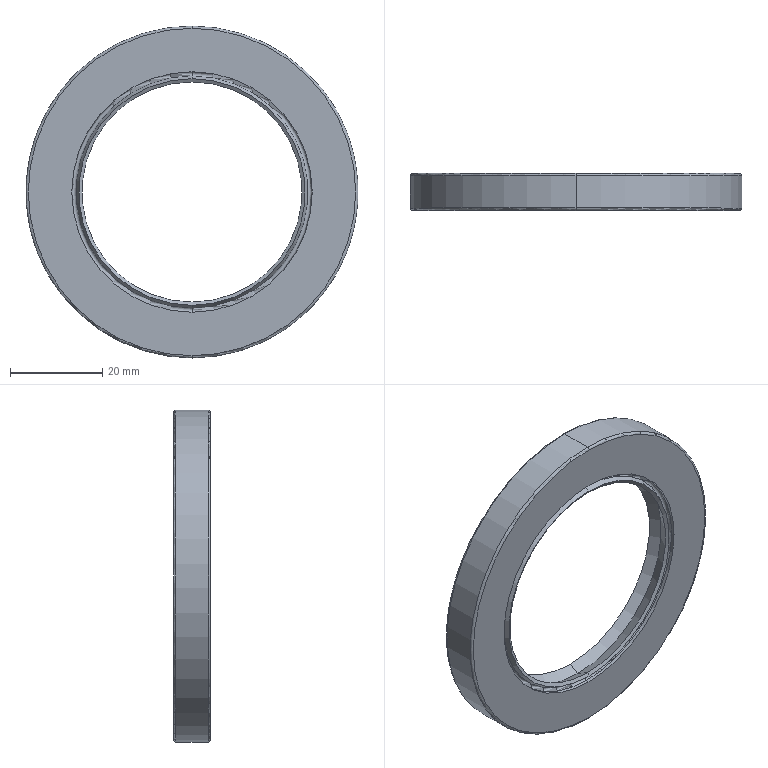Part | SolidWorks | features BaseBody 1 | 1 solid | 36 faces | box 72 x 8 x 72 mm | volume 7067 mm3 | torus 14 | cone 10 | cylinder 8 | plane 4 | commonest cylinder face diameters 52.145 x2 53.98 x2 69 x2 72 x2
STEP:
#1=CARTESIAN_POINT('',(0.,0.,24.573));
#2=VERTEX_POINT('',#1);
#3=CARTESIAN_POINT('',(0.,0.,-24.573));
#4=VERTEX_POINT('',#3);
#5=CARTESIAN_POINT('',(0.,0.,0.));
#6=DIRECTION('',(0.,1.,0.));
#7=DIRECTION('',(0.,0.,1.));
#8=AXIS2_PLACEMENT_3D('',#5,#6,#7);
#9=CIRCLE('',#8,24.573);
#10=EDGE_CURVE('',#2,#4,#9,.T.);
#11=ORIENTED_EDGE('',*,*,#10,.T.);
#12=CARTESIAN_POINT('',(0.,0.9821,-25.14));
#13=VERTEX_POINT('',#12);
#14=CARTESIAN_POINT('',(0.,0.9821,-25.14));
#15=DIRECTION('',(0.,0.866,-0.5));
#16=VECTOR('',#15,1000.);
#17=LINE('',#14,#16);
#18=EDGE_CURVE('',#4,#13,#17,.T.);
#19=ORIENTED_EDGE('',*,*,#18,.T.);
#20=CARTESIAN_POINT('',(0.,0.9821,25.14));
#21=VERTEX_POINT('',#20);
#22=CARTESIAN_POINT('',(0.,0.9821,0.));
#23=DIRECTION('',(0.,1.,0.));
#24=DIRECTION('',(0.,0.,1.));
#25=AXIS2_PLACEMENT_3D('',#22,#23,#24);
#26=CIRCLE('',#25,25.14);
#27=EDGE_CURVE('',#21,#13,#26,.T.);
#28=ORIENTED_EDGE('',*,*,#27,.F.);
#29=CARTESIAN_POINT('',(0.,0.9821,25.14));
#30=DIRECTION('',(0.,0.866,0.5));
#31=VECTOR('',#30,1000.);
#32=LINE('',#29,#31);
#33=EDGE_CURVE('',#2,#21,#32,.T.);
#34=ORIENTED_EDGE('',*,*,#33,.F.);
#35=EDGE_LOOP('',(#11,#19,#28,#34));
#36=FACE_OUTER_BOUND('',#35,.T.);
#37=CARTESIAN_POINT('',(0.,0.9821,0.));
#38=DIRECTION('',(0.,1.,0.));
#39=DIRECTION('',(0.,0.,1.));
#40=AXIS2_PLACEMENT_3D('',#37,#38,#39);
#41=CONICAL_SURFACE('',#40,25.14,0.5236);
#42=ADVANCED_FACE('',(#36),#41,.T.);
#43=CARTESIAN_POINT('',(0.,0.4041,-23.873));
#44=VERTEX_POINT('',#43);
#45=CARTESIAN_POINT('',(0.,0.4041,23.873));
#46=VERTEX_POINT('',#45);
#47=CARTESIAN_POINT('',(0.,0.4041,0.));
#48=DIRECTION('',(0.,1.,0.));
#49=DIRECTION('',(0.,0.,1.));
#50=AXIS2_PLACEMENT_3D('',#47,#48,#49);
#51=CIRCLE('',#50,23.873);
#52=EDGE_CURVE('',#44,#46,#51,.T.);
#53=ORIENTED_EDGE('',*,*,#52,.T.);
#54=CARTESIAN_POINT('',(0.,0.,24.573));
#55=DIRECTION('',(0.,-0.5,0.866));
#56=VECTOR('',#55,1000.);
#57=LINE('',#54,#56);
#58=EDGE_CURVE('',#46,#2,#57,.T.);
#59=ORIENTED_EDGE('',*,*,#58,.T.);
#60=CARTESIAN_POINT('',(0.,0.,0.));
#61=DIRECTION('',(0.,1.,0.));
#62=DIRECTION('',(0.,0.,1.));
#63=AXIS2_PLACEMENT_3D('',#60,#61,#62);
#64=CIRCLE('',#63,24.573);
#65=EDGE_CURVE('',#4,#2,#64,.T.);
#66=ORIENTED_EDGE('',*,*,#65,.F.);
#67=CARTESIAN_POINT('',(0.,0.,-24.573));
#68=DIRECTION('',(0.,-0.5,-0.866));
#69=VECTOR('',#68,1000.);
#70=LINE('',#67,#69);
#71=EDGE_CURVE('',#44,#4,#70,.T.);
#72=ORIENTED_EDGE('',*,*,#71,.F.);
#73=EDGE_LOOP('',(#53,#59,#66,#72));
#74=FACE_OUTER_BOUND('',#73,.T.);
#75=CARTESIAN_POINT('',(0.,0.,0.));
#76=DIRECTION('',(0.,-1.,0.));
#77=DIRECTION('',(0.,0.,-1.));
#78=AXIS2_PLACEMENT_3D('',#75,#76,#77);
#79=CONICAL_SURFACE('',#78,24.573,1.047);
#80=ADVANCED_FACE('',(#74),#79,.F.);
#81=ORIENTED_EDGE('',*,*,#52,.F.);
#82=CARTESIAN_POINT('',(0.,3.472,-25.644));
#83=VERTEX_POINT('',#82);
#84=CARTESIAN_POINT('',(0.,0.4041,-23.873));
#85=DIRECTION('',(0.,0.866,-0.5));
#86=VECTOR('',#85,1000.);
#87=LINE('',#84,#86);
#88=EDGE_CURVE('',#44,#83,#87,.T.);
#89=ORIENTED_EDGE('',*,*,#88,.T.);
#90=CARTESIAN_POINT('',(0.,3.472,25.644));
#91=VERTEX_POINT('',#90);
#92=CARTESIAN_POINT('',(0.,3.472,0.));
#93=DIRECTION('',(0.,1.,0.));
#94=DIRECTION('',(0.,0.,1.));
#95=AXIS2_PLACEMENT_3D('',#92,#93,#94);
#96=CIRCLE('',#95,25.644);
#97=EDGE_CURVE('',#83,#91,#96,.T.);
#98=ORIENTED_EDGE('',*,*,#97,.T.);
#99=CARTESIAN_POINT('',(0.,0.4041,23.873));
#100=DIRECTION('',(0.,0.866,0.5));
#101=VECTOR('',#100,1000.);
#102=LINE('',#99,#101);
#103=EDGE_CURVE('',#46,#91,#102,.T.);
#104=ORIENTED_EDGE('',*,*,#103,.F.);
#105=EDGE_LOOP('',(#81,#89,#98,#104));
#106=FACE_OUTER_BOUND('',#105,.T.);
#107=CARTESIAN_POINT('',(0.,0.4041,0.));
#108=DIRECTION('',(0.,1.,0.));
#109=DIRECTION('',(0.,0.,1.));
#110=AXIS2_PLACEMENT_3D('',#107,#108,#109);
#111=CONICAL_SURFACE('',#110,23.873,0.5236);
#112=ADVANCED_FACE('',(#106),#111,.F.);
#113=CARTESIAN_POINT('',(0.,5.7,-24.25));
#114=VERTEX_POINT('',#113);
#115=CARTESIAN_POINT('',(0.,5.7,24.25));
#116=VERTEX_POINT('',#115);
#117=CARTESIAN_POINT('',(0.,5.7,0.));
#118=DIRECTION('',(0.,1.,0.));
#119=DIRECTION('',(0.,0.,1.));
#120=AXIS2_PLACEMENT_3D('',#117,#118,#119);
#121=CIRCLE('',#120,24.25);
#122=EDGE_CURVE('',#114,#116,#121,.T.);
#123=ORIENTED_EDGE('',*,*,#122,.T.);
#124=CARTESIAN_POINT('',(0.,3.472,25.644));
#125=DIRECTION('',(0.,-0.8478,0.5303));
#126=VECTOR('',#125,1000.);
#127=LINE('',#124,#126);
#128=EDGE_CURVE('',#116,#91,#127,.T.);
#129=ORIENTED_EDGE('',*,*,#128,.T.);
#130=ORIENTED_EDGE('',*,*,#97,.F.);
#131=CARTESIAN_POINT('',(0.,3.472,-25.644));
#132=DIRECTION('',(0.,-0.8478,-0.5303));
#133=VECTOR('',#132,1000.);
#134=LINE('',#131,#133);
#135=EDGE_CURVE('',#114,#83,#134,.T.);
#136=ORIENTED_EDGE('',*,*,#135,.F.);
#137=EDGE_LOOP('',(#123,#129,#130,#136));
#138=FACE_OUTER_BOUND('',#137,.T.);
#139=CARTESIAN_POINT('',(0.,3.472,0.));
#140=DIRECTION('',(0.,-1.,0.));
#141=DIRECTION('',(0.,0.,-1.));
#142=AXIS2_PLACEMENT_3D('',#139,#140,#141);
#143=CONICAL_SURFACE('',#142,25.644,0.5589);
#144=ADVANCED_FACE('',(#138),#143,.F.);
#145=ORIENTED_EDGE('',*,*,#122,.F.);
#146=CARTESIAN_POINT('',(0.,7.,-26.328));
#147=VERTEX_POINT('',#146);
#148=CARTESIAN_POINT('',(0.,5.7,-24.25));
#149=DIRECTION('',(0.,0.5303,-0.8478));
#150=VECTOR('',#149,1000.);
#151=LINE('',#148,#150);
#152=EDGE_CURVE('',#114,#147,#151,.T.);
#153=ORIENTED_EDGE('',*,*,#152,.T.);
#154=CARTESIAN_POINT('',(0.,7.,26.328));
#155=VERTEX_POINT('',#154);
#156=CARTESIAN_POINT('',(0.,7.,0.));
#157=DIRECTION('',(0.,1.,0.));
#158=DIRECTION('',(0.,0.,1.));
#159=AXIS2_PLACEMENT_3D('',#156,#157,#158);
#160=CIRCLE('',#159,26.328);
#161=EDGE_CURVE('',#147,#155,#160,.T.);
#162=ORIENTED_EDGE('',*,*,#161,.T.);
#163=CARTESIAN_POINT('',(0.,5.7,24.25));
#164=DIRECTION('',(0.,0.5303,0.8478));
#165=VECTOR('',#164,1000.);
#166=LINE('',#163,#165);
#167=EDGE_CURVE('',#116,#155,#166,.T.);
#168=ORIENTED_EDGE('',*,*,#167,.F.);
#169=EDGE_LOOP('',(#145,#153,#162,#168));
#170=FACE_OUTER_BOUND('',#169,.T.);
#171=CARTESIAN_POINT('',(0.,5.7,0.));
#172=DIRECTION('',(0.,1.,0.));
#173=DIRECTION('',(0.,0.,1.));
#174=AXIS2_PLACEMENT_3D('',#171,#172,#173);
#175=CONICAL_SURFACE('',#174,24.25,1.012);
#176=ADVANCED_FACE('',(#170),#175,.F.);
#177=CARTESIAN_POINT('',(0.,5.981,26.99));
#178=VERTEX_POINT('',#177);
#179=CARTESIAN_POINT('',(0.,5.981,-26.99));
#180=VERTEX_POINT('',#179);
#181=CARTESIAN_POINT('',(0.,5.981,0.));
#182=DIRECTION('',(0.,1.,0.));
#183=DIRECTION('',(0.,0.,1.));
#184=AXIS2_PLACEMENT_3D('',#181,#182,#183);
#185=CIRCLE('',#184,26.99);
#186=EDGE_CURVE('',#178,#180,#185,.T.);
#187=ORIENTED_EDGE('',*,*,#186,.T.);
#188=CARTESIAN_POINT('',(0.,7.,-26.99));
#189=VERTEX_POINT('',#188);
#190=CARTESIAN_POINT('',(0.,6.49,-26.99));
#191=DIRECTION('',(1.,0.,0.));
#192=DIRECTION('',(0.,0.,-1.));
#193=AXIS2_PLACEMENT_3D('',#190,#191,#192);
#194=CIRCLE('',#193,0.5097);
#195=EDGE_CURVE('',#180,#189,#194,.T.);
#196=ORIENTED_EDGE('',*,*,#195,.T.);
#197=CARTESIAN_POINT('',(0.,7.,26.99));
#198=VERTEX_POINT('',#197);
#199=CARTESIAN_POINT('',(0.,7.,0.));
#200=DIRECTION('',(0.,1.,0.));
#201=DIRECTION('',(0.,0.,1.));
#202=AXIS2_PLACEMENT_3D('',#199,#200,#201);
#203=CIRCLE('',#202,26.99);
#204=EDGE_CURVE('',#198,#189,#203,.T.);
#205=ORIENTED_EDGE('',*,*,#204,.F.);
#206=CARTESIAN_POINT('',(0.,6.49,26.99));
#207=DIRECTION('',(-1.,0.,0.));
#208=DIRECTION('',(0.,0.,1.));
#209=AXIS2_PLACEMENT_3D('',#206,#207,#208);
#210=CIRCLE('',#209,0.5097);
#211=EDGE_CURVE('',#178,#198,#210,.T.);
#212=ORIENTED_EDGE('',*,*,#211,.F.);
#213=EDGE_LOOP('',(#187,#196,#205,#212));
#214=FACE_OUTER_BOUND('',#213,.T.);
#215=CARTESIAN_POINT('',(0.,6.49,0.));
#216=DIRECTION('',(0.,1.,0.));
#217=DIRECTION('',(0.,0.,1.));
#218=AXIS2_PLACEMENT_3D('',#215,#216,#217);
#219=TOROIDAL_SURFACE('',#218,26.99,0.5097);
#220=ADVANCED_FACE('',(#214),#219,.T.);
#221=CARTESIAN_POINT('',(0.,2.,26.99));
#222=VERTEX_POINT('',#221);
#223=CARTESIAN_POINT('',(0.,2.,-26.99));
#224=VERTEX_POINT('',#223);
#225=CARTESIAN_POINT('',(0.,2.,0.));
#226=DIRECTION('',(0.,1.,0.));
#227=DIRECTION('',(0.,0.,1.));
#228=AXIS2_PLACEMENT_3D('',#225,#226,#227);
#229=CIRCLE('',#228,26.99);
#230=EDGE_CURVE('',#222,#224,#229,.T.);
#231=ORIENTED_EDGE('',*,*,#230,.T.);
#232=CARTESIAN_POINT('',(0.,56.385,-26.99));
#233=DIRECTION('',(0.,1.,0.));
#234=VECTOR('',#233,1000.);
#235=LINE('',#232,#234);
#236=EDGE_CURVE('',#224,#180,#235,.T.);
#237=ORIENTED_EDGE('',*,*,#236,.T.);
#238=ORIENTED_EDGE('',*,*,#186,.F.);
#239=CARTESIAN_POINT('',(0.,56.385,26.99));
#240=DIRECTION('',(0.,1.,0.));
#241=VECTOR('',#240,1000.);
#242=LINE('',#239,#241);
#243=EDGE_CURVE('',#222,#178,#242,.T.);
#244=ORIENTED_EDGE('',*,*,#243,.F.);
#245=EDGE_LOOP('',(#231,#237,#238,#244));
#246=FACE_OUTER_BOUND('',#245,.T.);
#247=CARTESIAN_POINT('',(0.,56.385,0.));
#248=DIRECTION('',(0.,1.,0.));
#249=DIRECTION('',(0.,0.,1.));
#250=AXIS2_PLACEMENT_3D('',#247,#248,#249);
#251=CYLINDRICAL_SURFACE('',#250,26.99);
#252=ADVANCED_FACE('',(#246),#251,.T.);
#253=CARTESIAN_POINT('',(0.,2.,0.));
#254=DIRECTION('',(0.,1.,0.));
#255=DIRECTION('',(0.,0.,1.));
#256=AXIS2_PLACEMENT_3D('',#253,#254,#255);
#257=CIRCLE('',#256,26.99);
#258=EDGE_CURVE('',#224,#222,#257,.T.);
#259=ORIENTED_EDGE('',*,*,#258,.F.);
#260=CARTESIAN_POINT('',(0.,1.5,-27.49));
#261=VERTEX_POINT('',#260);
#262=CARTESIAN_POINT('',(0.,2.,-27.49));
#263=DIRECTION('',(1.,0.,0.));
#264=DIRECTION('',(0.,0.,-1.));
#265=AXIS2_PLACEMENT_3D('',#262,#263,#264);
#266=CIRCLE('',#265,0.5);
#267=EDGE_CURVE('',#224,#261,#266,.T.);
#268=ORIENTED_EDGE('',*,*,#267,.T.);
#269=CARTESIAN_POINT('',(0.,1.5,27.49));
#270=VERTEX_POINT('',#269);
#271=CARTESIAN_POINT('',(0.,1.5,0.));
#272=DIRECTION('',(0.,1.,0.));
#273=DIRECTION('',(0.,0.,1.));
#274=AXIS2_PLACEMENT_3D('',#271,#272,#273);
#275=CIRCLE('',#274,27.49);
#276=EDGE_CURVE('',#261,#270,#275,.T.);
#277=ORIENTED_EDGE('',*,*,#276,.T.);
#278=CARTESIAN_POINT('',(0.,2.,27.49));
#279=DIRECTION('',(-1.,0.,0.));
#280=DIRECTION('',(0.,0.,1.));
#281=AXIS2_PLACEMENT_3D('',#278,#279,#280);
#282=CIRCLE('',#281,0.5);
#283=EDGE_CURVE('',#222,#270,#282,.T.);
#284=ORIENTED_EDGE('',*,*,#283,.F.);
#285=EDGE_LOOP('',(#259,#268,#277,#284));
#286=FACE_OUTER_BOUND('',#285,.T.);
#287=CARTESIAN_POINT('',(0.,2.,0.));
#288=DIRECTION('',(0.,1.,0.));
#289=DIRECTION('',(0.,0.,1.));
#290=AXIS2_PLACEMENT_3D('',#287,#288,#289);
#291=TOROIDAL_SURFACE('',#290,27.49,0.5);
#292=ADVANCED_FACE('',(#286),#291,.F.);
#293=CARTESIAN_POINT('',(0.,1.5,-34.));
#294=VERTEX_POINT('',#293);
#295=CARTESIAN_POINT('',(0.,1.5,34.));
#296=VERTEX_POINT('',#295);
#297=CARTESIAN_POINT('',(0.,1.5,0.));
#298=DIRECTION('',(0.,1.,0.));
#299=DIRECTION('',(0.,0.,1.));
#300=AXIS2_PLACEMENT_3D('',#297,#298,#299);
#301=CIRCLE('',#300,34.);
#302=EDGE_CURVE('',#294,#296,#301,.T.);
#303=ORIENTED_EDGE('',*,*,#302,.F.);
#304=CARTESIAN_POINT('',(0.,2.,-34.5));
#305=VERTEX_POINT('',#304);
#306=CARTESIAN_POINT('',(0.,2.,-34.));
#307=DIRECTION('',(1.,0.,0.));
#308=DIRECTION('',(0.,0.,-1.));
#309=AXIS2_PLACEMENT_3D('',#306,#307,#308);
#310=CIRCLE('',#309,0.5);
#311=EDGE_CURVE('',#294,#305,#310,.T.);
#312=ORIENTED_EDGE('',*,*,#311,.T.);
#313=CARTESIAN_POINT('',(0.,2.,34.5));
#314=VERTEX_POINT('',#313);
#315=CARTESIAN_POINT('',(0.,2.,0.));
#316=DIRECTION('',(0.,1.,0.));
#317=DIRECTION('',(0.,0.,1.));
#318=AXIS2_PLACEMENT_3D('',#315,#316,#317);
#319=CIRCLE('',#318,34.5);
#320=EDGE_CURVE('',#305,#314,#319,.T.);
#321=ORIENTED_EDGE('',*,*,#320,.T.);
#322=CARTESIAN_POINT('',(0.,2.,34.));
#323=DIRECTION('',(-1.,0.,0.));
#324=DIRECTION('',(0.,0.,1.));
#325=AXIS2_PLACEMENT_3D('',#322,#323,#324);
#326=CIRCLE('',#325,0.5);
#327=EDGE_CURVE('',#296,#314,#326,.T.);
#328=ORIENTED_EDGE('',*,*,#327,.F.);
#329=EDGE_LOOP('',(#303,#312,#321,#328));
#330=FACE_OUTER_BOUND('',#329,.T.);
#331=CARTESIAN_POINT('',(0.,2.,0.));
#332=DIRECTION('',(0.,1.,0.));
#333=DIRECTION('',(0.,0.,1.));
#334=AXIS2_PLACEMENT_3D('',#331,#332,#333);
#335=TOROIDAL_SURFACE('',#334,34.,0.5);
#336=ADVANCED_FACE('',(#330),#335,.F.);
#337=ORIENTED_EDGE('',*,*,#320,.F.);
#338=CARTESIAN_POINT('',(0.,7.5,-34.5));
#339=VERTEX_POINT('',#338);
#340=CARTESIAN_POINT('',(0.,56.385,-34.5));
#341=DIRECTION('',(0.,1.,0.));
#342=VECTOR('',#341,1000.);
#343=LINE('',#340,#342);
#344=EDGE_CURVE('',#305,#339,#343,.T.);
#345=ORIENTED_EDGE('',*,*,#344,.T.);
#346=CARTESIAN_POINT('',(0.,7.5,34.5));
#347=VERTEX_POINT('',#346);
#348=CARTESIAN_POINT('',(0.,7.5,0.));
#349=DIRECTION('',(0.,1.,0.));
#350=DIRECTION('',(0.,0.,1.));
#351=AXIS2_PLACEMENT_3D('',#348,#349,#350);
#352=CIRCLE('',#351,34.5);
#353=EDGE_CURVE('',#339,#347,#352,.T.);
#354=ORIENTED_EDGE('',*,*,#353,.T.);
#355=CARTESIAN_POINT('',(0.,56.385,34.5));
#356=DIRECTION('',(0.,1.,0.));
#357=VECTOR('',#356,1000.);
#358=LINE('',#355,#357);
#359=EDGE_CURVE('',#314,#347,#358,.T.);
#360=ORIENTED_EDGE('',*,*,#359,.F.);
#361=EDGE_LOOP('',(#337,#345,#354,#360));
#362=FACE_OUTER_BOUND('',#361,.T.);
#363=CARTESIAN_POINT('',(0.,56.385,0.));
#364=DIRECTION('',(0.,1.,0.));
#365=DIRECTION('',(0.,0.,1.));
#366=AXIS2_PLACEMENT_3D('',#363,#364,#365);
#367=CYLINDRICAL_SURFACE('',#366,34.5);
#368=ADVANCED_FACE('',(#362),#367,.F.);
#369=CARTESIAN_POINT('',(0.,8.,35.));
#370=VERTEX_POINT('',#369);
#371=CARTESIAN_POINT('',(0.,8.,-35.));
#372=VERTEX_POINT('',#371);
#373=CARTESIAN_POINT('',(0.,8.,0.));
#374=DIRECTION('',(0.,1.,0.));
#375=DIRECTION('',(0.,0.,1.));
#376=AXIS2_PLACEMENT_3D('',#373,#374,#375);
#377=CIRCLE('',#376,35.);
#378=EDGE_CURVE('',#370,#372,#377,.T.);
#379=ORIENTED_EDGE('',*,*,#378,.T.);
#380=CARTESIAN_POINT('',(0.,7.5,-35.));
#381=DIRECTION('',(1.,0.,0.));
#382=DIRECTION('',(0.,0.,-1.));
#383=AXIS2_PLACEMENT_3D('',#380,#381,#382);
#384=CIRCLE('',#383,0.5);
#385=EDGE_CURVE('',#372,#339,#384,.T.);
#386=ORIENTED_EDGE('',*,*,#385,.T.);
#387=CARTESIAN_POINT('',(0.,7.5,0.));
#388=DIRECTION('',(0.,1.,0.));
#389=DIRECTION('',(0.,0.,1.));
#390=AXIS2_PLACEMENT_3D('',#387,#388,#389);
#391=CIRCLE('',#390,34.5);
#392=EDGE_CURVE('',#347,#339,#391,.T.);
#393=ORIENTED_EDGE('',*,*,#392,.F.);
#394=CARTESIAN_POINT('',(0.,7.5,35.));
#395=DIRECTION('',(-1.,0.,0.));
#396=DIRECTION('',(0.,0.,1.));
#397=AXIS2_PLACEMENT_3D('',#394,#395,#396);
#398=CIRCLE('',#397,0.5);
#399=EDGE_CURVE('',#370,#347,#398,.T.);
#400=ORIENTED_EDGE('',*,*,#399,.F.);
#401=EDGE_LOOP('',(#379,#386,#393,#400));
#402=FACE_OUTER_BOUND('',#401,.T.);
#403=CARTESIAN_POINT('',(0.,7.5,0.));
#404=DIRECTION('',(0.,1.,0.));
#405=DIRECTION('',(0.,0.,1.));
#406=AXIS2_PLACEMENT_3D('',#403,#404,#405);
#407=TOROIDAL_SURFACE('',#406,35.,0.5);
#408=ADVANCED_FACE('',(#402),#407,.T.);
#409=CARTESIAN_POINT('',(0.,7.5,36.));
#410=VERTEX_POINT('',#409);
#411=CARTESIAN_POINT('',(0.,7.5,-36.));
#412=VERTEX_POINT('',#411);
#413=CARTESIAN_POINT('',(0.,7.5,0.));
#414=DIRECTION('',(0.,1.,0.));
#415=DIRECTION('',(0.,0.,1.));
#416=AXIS2_PLACEMENT_3D('',#413,#414,#415);
#417=CIRCLE('',#416,36.);
#418=EDGE_CURVE('',#410,#412,#417,.T.);
#419=ORIENTED_EDGE('',*,*,#418,.T.);
#420=CARTESIAN_POINT('',(0.,8.,-35.5));
#421=VERTEX_POINT('',#420);
#422=CARTESIAN_POINT('',(0.,7.5,-35.5));
#423=DIRECTION('',(1.,0.,0.));
#424=DIRECTION('',(0.,0.,-1.));
#425=AXIS2_PLACEMENT_3D('',#422,#423,#424);
#426=CIRCLE('',#425,0.5);
#427=EDGE_CURVE('',#412,#421,#426,.T.);
#428=ORIENTED_EDGE('',*,*,#427,.T.);
#429=CARTESIAN_POINT('',(0.,8.,35.5));
#430=VERTEX_POINT('',#429);
#431=CARTESIAN_POINT('',(0.,8.,0.));
#432=DIRECTION('',(0.,1.,0.));
#433=DIRECTION('',(0.,0.,1.));
#434=AXIS2_PLACEMENT_3D('',#431,#432,#433);
#435=CIRCLE('',#434,35.5);
#436=EDGE_CURVE('',#430,#421,#435,.T.);
#437=ORIENTED_EDGE('',*,*,#436,.F.);
#438=CARTESIAN_POINT('',(0.,7.5,35.5));
#439=DIRECTION('',(-1.,0.,0.));
#440=DIRECTION('',(0.,0.,1.));
#441=AXIS2_PLACEMENT_3D('',#438,#439,#440);
#442=CIRCLE('',#441,0.5);
#443=EDGE_CURVE('',#410,#430,#442,.T.);
#444=ORIENTED_EDGE('',*,*,#443,.F.);
#445=EDGE_LOOP('',(#419,#428,#437,#444));
#446=FACE_OUTER_BOUND('',#445,.T.);
#447=CARTESIAN_POINT('',(0.,7.5,0.));
#448=DIRECTION('',(0.,1.,0.));
#449=DIRECTION('',(0.,0.,1.));
#450=AXIS2_PLACEMENT_3D('',#447,#448,#449);
#451=TOROIDAL_SURFACE('',#450,35.5,0.5);
#452=ADVANCED_FACE('',(#446),#451,.T.);
#453=CARTESIAN_POINT('',(0.,0.5,36.));
#454=VERTEX_POINT('',#453);
#455=CARTESIAN_POINT('',(0.,0.5,-36.));
#456=VERTEX_POINT('',#455);
#457=CARTESIAN_POINT('',(0.,0.5,0.));
#458=DIRECTION('',(0.,1.,0.));
#459=DIRECTION('',(0.,0.,1.));
#460=AXIS2_PLACEMENT_3D('',#457,#458,#459);
#461=CIRCLE('',#460,36.);
#462=EDGE_CURVE('',#454,#456,#461,.T.);
#463=ORIENTED_EDGE('',*,*,#462,.T.);
#464=CARTESIAN_POINT('',(0.,56.385,-36.));
#465=DIRECTION('',(0.,1.,0.));
#466=VECTOR('',#465,1000.);
#467=LINE('',#464,#466);
#468=EDGE_CURVE('',#456,#412,#467,.T.);
#469=ORIENTED_EDGE('',*,*,#468,.T.);
#470=ORIENTED_EDGE('',*,*,#418,.F.);
#471=CARTESIAN_POINT('',(0.,56.385,36.));
#472=DIRECTION('',(0.,1.,0.));
#473=VECTOR('',#472,1000.);
#474=LINE('',#471,#473);
#475=EDGE_CURVE('',#454,#410,#474,.T.);
#476=ORIENTED_EDGE('',*,*,#475,.F.);
#477=EDGE_LOOP('',(#463,#469,#470,#476));
#478=FACE_OUTER_BOUND('',#477,.T.);
#479=CARTESIAN_POINT('',(0.,56.385,0.));
#480=DIRECTION('',(0.,1.,0.));
#481=DIRECTION('',(0.,0.,1.));
#482=AXIS2_PLACEMENT_3D('',#479,#480,#481);
#483=CYLINDRICAL_SURFACE('',#482,36.);
#484=ADVANCED_FACE('',(#478),#483,.T.);
#485=CARTESIAN_POINT('',(0.,0.,35.5));
#486=VERTEX_POINT('',#485);
#487=CARTESIAN_POINT('',(0.,0.,-35.5));
#488=VERTEX_POINT('',#487);
#489=CARTESIAN_POINT('',(0.,0.,0.));
#490=DIRECTION('',(0.,1.,0.));
#491=DIRECTION('',(0.,0.,1.));
#492=AXIS2_PLACEMENT_3D('',#489,#490,#491);
#493=CIRCLE('',#492,35.5);
#494=EDGE_CURVE('',#486,#488,#493,.T.);
#495=ORIENTED_EDGE('',*,*,#494,.T.);
#496=CARTESIAN_POINT('',(0.,0.5,-35.5));
#497=DIRECTION('',(1.,0.,0.));
#498=DIRECTION('',(0.,0.,-1.));
#499=AXIS2_PLACEMENT_3D('',#496,#497,#498);
#500=CIRCLE('',#499,0.5);
#501=EDGE_CURVE('',#488,#456,#500,.T.);
#502=ORIENTED_EDGE('',*,*,#501,.T.);
#503=ORIENTED_EDGE('',*,*,#462,.F.);
#504=CARTESIAN_POINT('',(0.,0.5,35.5));
#505=DIRECTION('',(-1.,0.,0.));
#506=DIRECTION('',(0.,0.,1.));
#507=AXIS2_PLACEMENT_3D('',#504,#505,#506);
#508=CIRCLE('',#507,0.5);
#509=EDGE_CURVE('',#486,#454,#508,.T.);
#510=ORIENTED_EDGE('',*,*,#509,.F.);
#511=EDGE_LOOP('',(#495,#502,#503,#510));
#512=FACE_OUTER_BOUND('',#511,.T.);
#513=CARTESIAN_POINT('',(0.,0.5,0.));
#514=DIRECTION('',(0.,1.,0.));
#515=DIRECTION('',(0.,0.,1.));
#516=AXIS2_PLACEMENT_3D('',#513,#514,#515);
#517=TOROIDAL_SURFACE('',#516,35.5,0.5);
#518=ADVANCED_FACE('',(#512),#517,.T.);
#519=CARTESIAN_POINT('',(0.,0.,-26.073));
#520=VERTEX_POINT('',#519);
#521=CARTESIAN_POINT('',(0.,0.,26.073));
#522=VERTEX_POINT('',#521);
#523=CARTESIAN_POINT('',(0.,0.,0.));
#524=DIRECTION('',(0.,1.,0.));
#525=DIRECTION('',(0.,0.,1.));
#526=AXIS2_PLACEMENT_3D('',#523,#524,#525);
#527=CIRCLE('',#526,26.073);
#528=EDGE_CURVE('',#520,#522,#527,.T.);
#529=ORIENTED_EDGE('',*,*,#528,.F.);
#530=CARTESIAN_POINT('',(0.,0.7321,-26.073));
#531=VERTEX_POINT('',#530);
#532=CARTESIAN_POINT('',(0.,56.385,-26.073));
#533=DIRECTION('',(0.,1.,0.));
#534=VECTOR('',#533,1000.);
#535=LINE('',#532,#534);
#536=EDGE_CURVE('',#520,#531,#535,.T.);
#537=ORIENTED_EDGE('',*,*,#536,.T.);
#538=CARTESIAN_POINT('',(0.,0.7321,26.073));
#539=VERTEX_POINT('',#538);
#540=CARTESIAN_POINT('',(0.,0.7321,0.));
#541=DIRECTION('',(0.,1.,0.));
#542=DIRECTION('',(0.,0.,1.));
#543=AXIS2_PLACEMENT_3D('',#540,#541,#542);
#544=CIRCLE('',#543,26.073);
#545=EDGE_CURVE('',#531,#539,#544,.T.);
#546=ORIENTED_EDGE('',*,*,#545,.T.);
#547=CARTESIAN_POINT('',(0.,56.385,26.073));
#548=DIRECTION('',(0.,1.,0.));
#549=VECTOR('',#548,1000.);
#550=LINE('',#547,#549);
#551=EDGE_CURVE('',#522,#539,#550,.T.);
#552=ORIENTED_EDGE('',*,*,#551,.F.);
#553=EDGE_LOOP('',(#529,#537,#546,#552));
#554=FACE_OUTER_BOUND('',#553,.T.);
#555=CARTESIAN_POINT('',(0.,56.385,0.));
#556=DIRECTION('',(0.,1.,0.));
#557=DIRECTION('',(0.,0.,1.));
#558=AXIS2_PLACEMENT_3D('',#555,#556,#557);
#559=CYLINDRICAL_SURFACE('',#558,26.073);
#560=ADVANCED_FACE('',(#554),#559,.F.);
#561=ORIENTED_EDGE('',*,*,#545,.F.);
#562=CARTESIAN_POINT('',(0.,0.7321,-25.573));
#563=DIRECTION('',(1.,0.,0.));
#564=DIRECTION('',(0.,0.,-1.));
#565=AXIS2_PLACEMENT_3D('',#562,#563,#564);
#566=CIRCLE('',#565,0.5);
#567=EDGE_CURVE('',#531,#13,#566,.T.);
#568=ORIENTED_EDGE('',*,*,#567,.T.);
#569=CARTESIAN_POINT('',(0.,0.9821,0.));
#570=DIRECTION('',(0.,1.,0.));
#571=DIRECTION('',(0.,0.,1.));
#572=AXIS2_PLACEMENT_3D('',#569,#570,#571);
#573=CIRCLE('',#572,25.14);
#574=EDGE_CURVE('',#13,#21,#573,.T.);
#575=ORIENTED_EDGE('',*,*,#574,.T.);
#576=CARTESIAN_POINT('',(0.,0.7321,25.573));
#577=DIRECTION('',(-1.,0.,0.));
#578=DIRECTION('',(0.,0.,1.));
#579=AXIS2_PLACEMENT_3D('',#576,#577,#578);
#580=CIRCLE('',#579,0.5);
#581=EDGE_CURVE('',#539,#21,#580,.T.);
#582=ORIENTED_EDGE('',*,*,#581,.F.);
#583=EDGE_LOOP('',(#561,#568,#575,#582));
#584=FACE_OUTER_BOUND('',#583,.T.);
#585=CARTESIAN_POINT('',(0.,0.7321,0.));
#586=DIRECTION('',(0.,1.,0.));
#587=DIRECTION('',(0.,0.,1.));
#588=AXIS2_PLACEMENT_3D('',#585,#586,#587);
#589=TOROIDAL_SURFACE('',#588,25.573,0.5);
#590=ADVANCED_FACE('',(#584),#589,.F.);
#591=CARTESIAN_POINT('',(0.,7.,0.));
#592=DIRECTION('',(0.,1.,0.));
#593=DIRECTION('',(0.,0.,1.));
#594=AXIS2_PLACEMENT_3D('',#591,#592,#593);
#595=CIRCLE('',#594,26.328);
#596=EDGE_CURVE('',#155,#147,#595,.T.);
#597=ORIENTED_EDGE('',*,*,#596,.F.);
#598=ORIENTED_EDGE('',*,*,#161,.F.);
#599=EDGE_LOOP('',(#597,#598));
#600=FACE_BOUND('',#599,.T.);
#601=ORIENTED_EDGE('',*,*,#204,.T.);
#602=CARTESIAN_POINT('',(0.,7.,0.));
#603=DIRECTION('',(0.,1.,0.));
#604=DIRECTION('',(0.,0.,1.));
#605=AXIS2_PLACEMENT_3D('',#602,#603,#604);
#606=CIRCLE('',#605,26.99);
#607=EDGE_CURVE('',#189,#198,#606,.T.);
#608=ORIENTED_EDGE('',*,*,#607,.T.);
#609=EDGE_LOOP('',(#601,#608));
#610=FACE_OUTER_BOUND('',#609,.T.);
#611=CARTESIAN_POINT('',(0.,7.,26.328));
#612=DIRECTION('',(0.,1.,0.));
#613=DIRECTION('',(1.,0.,0.));
#614=AXIS2_PLACEMENT_3D('',#611,#612,#613);
#615=PLANE('',#614);
#616=ADVANCED_FACE('',(#600,#610),#615,.T.);
#617=CARTESIAN_POINT('',(0.,1.5,0.));
#618=DIRECTION('',(0.,1.,0.));
#619=DIRECTION('',(0.,0.,1.));
#620=AXIS2_PLACEMENT_3D('',#617,#618,#619);
#621=CIRCLE('',#620,27.49);
#622=EDGE_CURVE('',#270,#261,#621,.T.);
#623=ORIENTED_EDGE('',*,*,#622,.F.);
#624=ORIENTED_EDGE('',*,*,#276,.F.);
#625=EDGE_LOOP('',(#623,#624));
#626=FACE_BOUND('',#625,.T.);
#627=CARTESIAN_POINT('',(0.,1.5,0.));
#628=DIRECTION('',(0.,1.,0.));
#629=DIRECTION('',(0.,0.,1.));
#630=AXIS2_PLACEMENT_3D('',#627,#628,#629);
#631=CIRCLE('',#630,34.);
#632=EDGE_CURVE('',#296,#294,#631,.T.);
#633=ORIENTED_EDGE('',*,*,#632,.T.);
#634=ORIENTED_EDGE('',*,*,#302,.T.);
#635=EDGE_LOOP('',(#633,#634));
#636=FACE_OUTER_BOUND('',#635,.T.);
#637=CARTESIAN_POINT('',(0.,1.5,34.));
#638=DIRECTION('',(0.,1.,0.));
#639=DIRECTION('',(1.,0.,0.));
#640=AXIS2_PLACEMENT_3D('',#637,#638,#639);
#641=PLANE('',#640);
#642=ADVANCED_FACE('',(#626,#636),#641,.T.);
#643=ORIENTED_EDGE('',*,*,#378,.F.);
#644=CARTESIAN_POINT('',(0.,8.,0.));
#645=DIRECTION('',(0.,1.,0.));
#646=DIRECTION('',(0.,0.,1.));
#647=AXIS2_PLACEMENT_3D('',#644,#645,#646);
#648=CIRCLE('',#647,35.);
#649=EDGE_CURVE('',#372,#370,#648,.T.);
#650=ORIENTED_EDGE('',*,*,#649,.F.);
#651=EDGE_LOOP('',(#643,#650));
#652=FACE_BOUND('',#651,.T.);
#653=ORIENTED_EDGE('',*,*,#436,.T.);
#654=CARTESIAN_POINT('',(0.,8.,0.));
#655=DIRECTION('',(0.,1.,0.));
#656=DIRECTION('',(0.,0.,1.));
#657=AXIS2_PLACEMENT_3D('',#654,#655,#656);
#658=CIRCLE('',#657,35.5);
#659=EDGE_CURVE('',#421,#430,#658,.T.);
#660=ORIENTED_EDGE('',*,*,#659,.T.);
#661=EDGE_LOOP('',(#653,#660));
#662=FACE_OUTER_BOUND('',#661,.T.);
#663=CARTESIAN_POINT('',(0.,8.,35.));
#664=DIRECTION('',(0.,1.,0.));
#665=DIRECTION('',(1.,0.,0.));
#666=AXIS2_PLACEMENT_3D('',#663,#664,#665);
#667=PLANE('',#666);
#668=ADVANCED_FACE('',(#652,#662),#667,.T.);
#669=CARTESIAN_POINT('',(0.,0.,0.));
#670=DIRECTION('',(0.,1.,0.));
#671=DIRECTION('',(0.,0.,1.));
#672=AXIS2_PLACEMENT_3D('',#669,#670,#671);
#673=CIRCLE('',#672,26.073);
#674=EDGE_CURVE('',#522,#520,#673,.T.);
#675=ORIENTED_EDGE('',*,*,#674,.T.);
#676=ORIENTED_EDGE('',*,*,#528,.T.);
#677=EDGE_LOOP('',(#675,#676));
#678=FACE_BOUND('',#677,.T.);
#679=ORIENTED_EDGE('',*,*,#494,.F.);
#680=CARTESIAN_POINT('',(0.,0.,0.));
#681=DIRECTION('',(0.,1.,0.));
#682=DIRECTION('',(0.,0.,1.));
#683=AXIS2_PLACEMENT_3D('',#680,#681,#682);
#684=CIRCLE('',#683,35.5);
#685=EDGE_CURVE('',#488,#486,#684,.T.);
#686=ORIENTED_EDGE('',*,*,#685,.F.);
#687=EDGE_LOOP('',(#679,#686));
#688=FACE_OUTER_BOUND('',#687,.T.);
#689=CARTESIAN_POINT('',(0.,0.,35.5));
#690=DIRECTION('',(0.,-1.,0.));
#691=DIRECTION('',(0.,0.,-1.));
#692=AXIS2_PLACEMENT_3D('',#689,#690,#691);
#693=PLANE('',#692);
#694=ADVANCED_FACE('',(#678,#688),#693,.T.);
#695=ORIENTED_EDGE('',*,*,#567,.F.);
#696=CARTESIAN_POINT('',(0.,0.7321,0.));
#697=DIRECTION('',(0.,1.,0.));
#698=DIRECTION('',(0.,0.,1.));
#699=AXIS2_PLACEMENT_3D('',#696,#697,#698);
#700=CIRCLE('',#699,26.073);
#701=EDGE_CURVE('',#539,#531,#700,.T.);
#702=ORIENTED_EDGE('',*,*,#701,.F.);
#703=ORIENTED_EDGE('',*,*,#581,.T.);
#704=ORIENTED_EDGE('',*,*,#27,.T.);
#705=EDGE_LOOP('',(#695,#702,#703,#704));
#706=FACE_OUTER_BOUND('',#705,.T.);
#707=CARTESIAN_POINT('',(0.,0.7321,0.));
#708=DIRECTION('',(0.,1.,0.));
#709=DIRECTION('',(0.,0.,1.));
#710=AXIS2_PLACEMENT_3D('',#707,#708,#709);
#711=TOROIDAL_SURFACE('',#710,25.573,0.5);
#712=ADVANCED_FACE('',(#706),#711,.F.);
#713=ORIENTED_EDGE('',*,*,#536,.F.);
#714=ORIENTED_EDGE('',*,*,#674,.F.);
#715=ORIENTED_EDGE('',*,*,#551,.T.);
#716=ORIENTED_EDGE('',*,*,#701,.T.);
#717=EDGE_LOOP('',(#713,#714,#715,#716));
#718=FACE_OUTER_BOUND('',#717,.T.);
#719=CARTESIAN_POINT('',(0.,56.385,0.));
#720=DIRECTION('',(0.,1.,0.));
#721=DIRECTION('',(0.,0.,1.));
#722=AXIS2_PLACEMENT_3D('',#719,#720,#721);
#723=CYLINDRICAL_SURFACE('',#722,26.073);
#724=ADVANCED_FACE('',(#718),#723,.F.);
#725=ORIENTED_EDGE('',*,*,#501,.F.);
#726=ORIENTED_EDGE('',*,*,#685,.T.);
#727=ORIENTED_EDGE('',*,*,#509,.T.);
#728=CARTESIAN_POINT('',(0.,0.5,0.));
#729=DIRECTION('',(0.,1.,0.));
#730=DIRECTION('',(0.,0.,1.));
#731=AXIS2_PLACEMENT_3D('',#728,#729,#730);
#732=CIRCLE('',#731,36.);
#733=EDGE_CURVE('',#456,#454,#732,.T.);
#734=ORIENTED_EDGE('',*,*,#733,.F.);
#735=EDGE_LOOP('',(#725,#726,#727,#734));
#736=FACE_OUTER_BOUND('',#735,.T.);
#737=CARTESIAN_POINT('',(0.,0.5,0.));
#738=DIRECTION('',(0.,1.,0.));
#739=DIRECTION('',(0.,0.,1.));
#740=AXIS2_PLACEMENT_3D('',#737,#738,#739);
#741=TOROIDAL_SURFACE('',#740,35.5,0.5);
#742=ADVANCED_FACE('',(#736),#741,.T.);
#743=ORIENTED_EDGE('',*,*,#468,.F.);
#744=ORIENTED_EDGE('',*,*,#733,.T.);
#745=ORIENTED_EDGE('',*,*,#475,.T.);
#746=CARTESIAN_POINT('',(0.,7.5,0.));
#747=DIRECTION('',(0.,1.,0.));
#748=DIRECTION('',(0.,0.,1.));
#749=AXIS2_PLACEMENT_3D('',#746,#747,#748);
#750=CIRCLE('',#749,36.);
#751=EDGE_CURVE('',#412,#410,#750,.T.);
#752=ORIENTED_EDGE('',*,*,#751,.F.);
#753=EDGE_LOOP('',(#743,#744,#745,#752));
#754=FACE_OUTER_BOUND('',#753,.T.);
#755=CARTESIAN_POINT('',(0.,56.385,0.));
#756=DIRECTION('',(0.,1.,0.));
#757=DIRECTION('',(0.,0.,1.));
#758=AXIS2_PLACEMENT_3D('',#755,#756,#757);
#759=CYLINDRICAL_SURFACE('',#758,36.);
#760=ADVANCED_FACE('',(#754),#759,.T.);
#761=ORIENTED_EDGE('',*,*,#427,.F.);
#762=ORIENTED_EDGE('',*,*,#751,.T.);
#763=ORIENTED_EDGE('',*,*,#443,.T.);
#764=ORIENTED_EDGE('',*,*,#659,.F.);
#765=EDGE_LOOP('',(#761,#762,#763,#764));
#766=FACE_OUTER_BOUND('',#765,.T.);
#767=CARTESIAN_POINT('',(0.,7.5,0.));
#768=DIRECTION('',(0.,1.,0.));
#769=DIRECTION('',(0.,0.,1.));
#770=AXIS2_PLACEMENT_3D('',#767,#768,#769);
#771=TOROIDAL_SURFACE('',#770,35.5,0.5);
#772=ADVANCED_FACE('',(#766),#771,.T.);
#773=ORIENTED_EDGE('',*,*,#385,.F.);
#774=ORIENTED_EDGE('',*,*,#649,.T.);
#775=ORIENTED_EDGE('',*,*,#399,.T.);
#776=ORIENTED_EDGE('',*,*,#353,.F.);
#777=EDGE_LOOP('',(#773,#774,#775,#776));
#778=FACE_OUTER_BOUND('',#777,.T.);
#779=CARTESIAN_POINT('',(0.,7.5,0.));
#780=DIRECTION('',(0.,1.,0.));
#781=DIRECTION('',(0.,0.,1.));
#782=AXIS2_PLACEMENT_3D('',#779,#780,#781);
#783=TOROIDAL_SURFACE('',#782,35.,0.5);
#784=ADVANCED_FACE('',(#778),#783,.T.);
#785=ORIENTED_EDGE('',*,*,#344,.F.);
#786=CARTESIAN_POINT('',(0.,2.,0.));
#787=DIRECTION('',(0.,1.,0.));
#788=DIRECTION('',(0.,0.,1.));
#789=AXIS2_PLACEMENT_3D('',#786,#787,#788);
#790=CIRCLE('',#789,34.5);
#791=EDGE_CURVE('',#314,#305,#790,.T.);
#792=ORIENTED_EDGE('',*,*,#791,.F.);
#793=ORIENTED_EDGE('',*,*,#359,.T.);
#794=ORIENTED_EDGE('',*,*,#392,.T.);
#795=EDGE_LOOP('',(#785,#792,#793,#794));
#796=FACE_OUTER_BOUND('',#795,.T.);
#797=CARTESIAN_POINT('',(0.,56.385,0.));
#798=DIRECTION('',(0.,1.,0.));
#799=DIRECTION('',(0.,0.,1.));
#800=AXIS2_PLACEMENT_3D('',#797,#798,#799);
#801=CYLINDRICAL_SURFACE('',#800,34.5);
#802=ADVANCED_FACE('',(#796),#801,.F.);
#803=ORIENTED_EDGE('',*,*,#311,.F.);
#804=ORIENTED_EDGE('',*,*,#632,.F.);
#805=ORIENTED_EDGE('',*,*,#327,.T.);
#806=ORIENTED_EDGE('',*,*,#791,.T.);
#807=EDGE_LOOP('',(#803,#804,#805,#806));
#808=FACE_OUTER_BOUND('',#807,.T.);
#809=CARTESIAN_POINT('',(0.,2.,0.));
#810=DIRECTION('',(0.,1.,0.));
#811=DIRECTION('',(0.,0.,1.));
#812=AXIS2_PLACEMENT_3D('',#809,#810,#811);
#813=TOROIDAL_SURFACE('',#812,34.,0.5);
#814=ADVANCED_FACE('',(#808),#813,.F.);
#815=ORIENTED_EDGE('',*,*,#267,.F.);
#816=ORIENTED_EDGE('',*,*,#230,.F.);
#817=ORIENTED_EDGE('',*,*,#283,.T.);
#818=ORIENTED_EDGE('',*,*,#622,.T.);
#819=EDGE_LOOP('',(#815,#816,#817,#818));
#820=FACE_OUTER_BOUND('',#819,.T.);
#821=CARTESIAN_POINT('',(0.,2.,0.));
#822=DIRECTION('',(0.,1.,0.));
#823=DIRECTION('',(0.,0.,1.));
#824=AXIS2_PLACEMENT_3D('',#821,#822,#823);
#825=TOROIDAL_SURFACE('',#824,27.49,0.5);
#826=ADVANCED_FACE('',(#820),#825,.F.);
#827=ORIENTED_EDGE('',*,*,#236,.F.);
#828=ORIENTED_EDGE('',*,*,#258,.T.);
#829=ORIENTED_EDGE('',*,*,#243,.T.);
#830=CARTESIAN_POINT('',(0.,5.981,0.));
#831=DIRECTION('',(0.,1.,0.));
#832=DIRECTION('',(0.,0.,1.));
#833=AXIS2_PLACEMENT_3D('',#830,#831,#832);
#834=CIRCLE('',#833,26.99);
#835=EDGE_CURVE('',#180,#178,#834,.T.);
#836=ORIENTED_EDGE('',*,*,#835,.F.);
#837=EDGE_LOOP('',(#827,#828,#829,#836));
#838=FACE_OUTER_BOUND('',#837,.T.);
#839=CARTESIAN_POINT('',(0.,56.385,0.));
#840=DIRECTION('',(0.,1.,0.));
#841=DIRECTION('',(0.,0.,1.));
#842=AXIS2_PLACEMENT_3D('',#839,#840,#841);
#843=CYLINDRICAL_SURFACE('',#842,26.99);
#844=ADVANCED_FACE('',(#838),#843,.T.);
#845=ORIENTED_EDGE('',*,*,#195,.F.);
#846=ORIENTED_EDGE('',*,*,#835,.T.);
#847=ORIENTED_EDGE('',*,*,#211,.T.);
#848=ORIENTED_EDGE('',*,*,#607,.F.);
#849=EDGE_LOOP('',(#845,#846,#847,#848));
#850=FACE_OUTER_BOUND('',#849,.T.);
#851=CARTESIAN_POINT('',(0.,6.49,0.));
#852=DIRECTION('',(0.,1.,0.));
#853=DIRECTION('',(0.,0.,1.));
#854=AXIS2_PLACEMENT_3D('',#851,#852,#853);
#855=TOROIDAL_SURFACE('',#854,26.99,0.5097);
#856=ADVANCED_FACE('',(#850),#855,.T.);
#857=ORIENTED_EDGE('',*,*,#152,.F.);
#858=CARTESIAN_POINT('',(0.,5.7,0.));
#859=DIRECTION('',(0.,1.,0.));
#860=DIRECTION('',(0.,0.,1.));
#861=AXIS2_PLACEMENT_3D('',#858,#859,#860);
#862=CIRCLE('',#861,24.25);
#863=EDGE_CURVE('',#116,#114,#862,.T.);
#864=ORIENTED_EDGE('',*,*,#863,.F.);
#865=ORIENTED_EDGE('',*,*,#167,.T.);
#866=ORIENTED_EDGE('',*,*,#596,.T.);
#867=EDGE_LOOP('',(#857,#864,#865,#866));
#868=FACE_OUTER_BOUND('',#867,.T.);
#869=CARTESIAN_POINT('',(0.,5.7,0.));
#870=DIRECTION('',(0.,1.,0.));
#871=DIRECTION('',(0.,0.,1.));
#872=AXIS2_PLACEMENT_3D('',#869,#870,#871);
#873=CONICAL_SURFACE('',#872,24.25,1.012);
#874=ADVANCED_FACE('',(#868),#873,.F.);
#875=ORIENTED_EDGE('',*,*,#128,.F.);
#876=ORIENTED_EDGE('',*,*,#863,.T.);
#877=ORIENTED_EDGE('',*,*,#135,.T.);
#878=CARTESIAN_POINT('',(0.,3.472,0.));
#879=DIRECTION('',(0.,1.,0.));
#880=DIRECTION('',(0.,0.,1.));
#881=AXIS2_PLACEMENT_3D('',#878,#879,#880);
#882=CIRCLE('',#881,25.644);
#883=EDGE_CURVE('',#91,#83,#882,.T.);
#884=ORIENTED_EDGE('',*,*,#883,.F.);
#885=EDGE_LOOP('',(#875,#876,#877,#884));
#886=FACE_OUTER_BOUND('',#885,.T.);
#887=CARTESIAN_POINT('',(0.,3.472,0.));
#888=DIRECTION('',(0.,-1.,0.));
#889=DIRECTION('',(0.,0.,-1.));
#890=AXIS2_PLACEMENT_3D('',#887,#888,#889);
#891=CONICAL_SURFACE('',#890,25.644,0.5589);
#892=ADVANCED_FACE('',(#886),#891,.F.);
#893=ORIENTED_EDGE('',*,*,#88,.F.);
#894=CARTESIAN_POINT('',(0.,0.4041,0.));
#895=DIRECTION('',(0.,1.,0.));
#896=DIRECTION('',(0.,0.,1.));
#897=AXIS2_PLACEMENT_3D('',#894,#895,#896);
#898=CIRCLE('',#897,23.873);
#899=EDGE_CURVE('',#46,#44,#898,.T.);
#900=ORIENTED_EDGE('',*,*,#899,.F.);
#901=ORIENTED_EDGE('',*,*,#103,.T.);
#902=ORIENTED_EDGE('',*,*,#883,.T.);
#903=EDGE_LOOP('',(#893,#900,#901,#902));
#904=FACE_OUTER_BOUND('',#903,.T.);
#905=CARTESIAN_POINT('',(0.,0.4041,0.));
#906=DIRECTION('',(0.,1.,0.));
#907=DIRECTION('',(0.,0.,1.));
#908=AXIS2_PLACEMENT_3D('',#905,#906,#907);
#909=CONICAL_SURFACE('',#908,23.873,0.5236);
#910=ADVANCED_FACE('',(#904),#909,.F.);
#911=ORIENTED_EDGE('',*,*,#58,.F.);
#912=ORIENTED_EDGE('',*,*,#899,.T.);
#913=ORIENTED_EDGE('',*,*,#71,.T.);
#914=ORIENTED_EDGE('',*,*,#10,.F.);
#915=EDGE_LOOP('',(#911,#912,#913,#914));
#916=FACE_OUTER_BOUND('',#915,.T.);
#917=CARTESIAN_POINT('',(0.,0.,0.));
#918=DIRECTION('',(0.,-1.,0.));
#919=DIRECTION('',(0.,0.,-1.));
#920=AXIS2_PLACEMENT_3D('',#917,#918,#919);
#921=CONICAL_SURFACE('',#920,24.573,1.047);
#922=ADVANCED_FACE('',(#916),#921,.F.);
#923=ORIENTED_EDGE('',*,*,#18,.F.);
#924=ORIENTED_EDGE('',*,*,#65,.T.);
#925=ORIENTED_EDGE('',*,*,#33,.T.);
#926=ORIENTED_EDGE('',*,*,#574,.F.);
#927=EDGE_LOOP('',(#923,#924,#925,#926));
#928=FACE_OUTER_BOUND('',#927,.T.);
#929=CARTESIAN_POINT('',(0.,0.9821,0.));
#930=DIRECTION('',(0.,1.,0.));
#931=DIRECTION('',(0.,0.,1.));
#932=AXIS2_PLACEMENT_3D('',#929,#930,#931);
#933=CONICAL_SURFACE('',#932,25.14,0.5236);
#934=ADVANCED_FACE('',(#928),#933,.T.);
#935=CLOSED_SHELL('',(#42,#80,#112,#144,#176,#220,#252,#292,#336,#368,#408,#452,#484,#518,#560,#590,#616,#642,#668,#694,#712,#724,#742,#760,#772,#784,#802,#814,#826,#844,#856,#874,#892,#910,#922,#934));
#936=MANIFOLD_SOLID_BREP('',#935);
#937=CARTESIAN_POINT('',(0.,0.,0.));
#938=DIRECTION('',(0.,0.,1.));
#939=DIRECTION('',(1.,0.,0.));
#940=AXIS2_PLACEMENT_3D('',#937,#938,#939);
#941=(LENGTH_UNIT()NAMED_UNIT(*)SI_UNIT(.MILLI.,.METRE.));
#942=UNCERTAINTY_MEASURE_WITH_UNIT(LENGTH_MEASURE(0.00001),#941,'','');
#943=(NAMED_UNIT(*)PLANE_ANGLE_UNIT()SI_UNIT($,.RADIAN.));
#944=(NAMED_UNIT(*)SI_UNIT($,.STERADIAN.)SOLID_ANGLE_UNIT());
#945=(GEOMETRIC_REPRESENTATION_CONTEXT(3)GLOBAL_UNCERTAINTY_ASSIGNED_CONTEXT((#942))GLOBAL_UNIT_ASSIGNED_CONTEXT((#941,#943,#944))REPRESENTATION_CONTEXT('',''));
#946=ADVANCED_BREP_SHAPE_REPRESENTATION('',(#936,#940),#945);